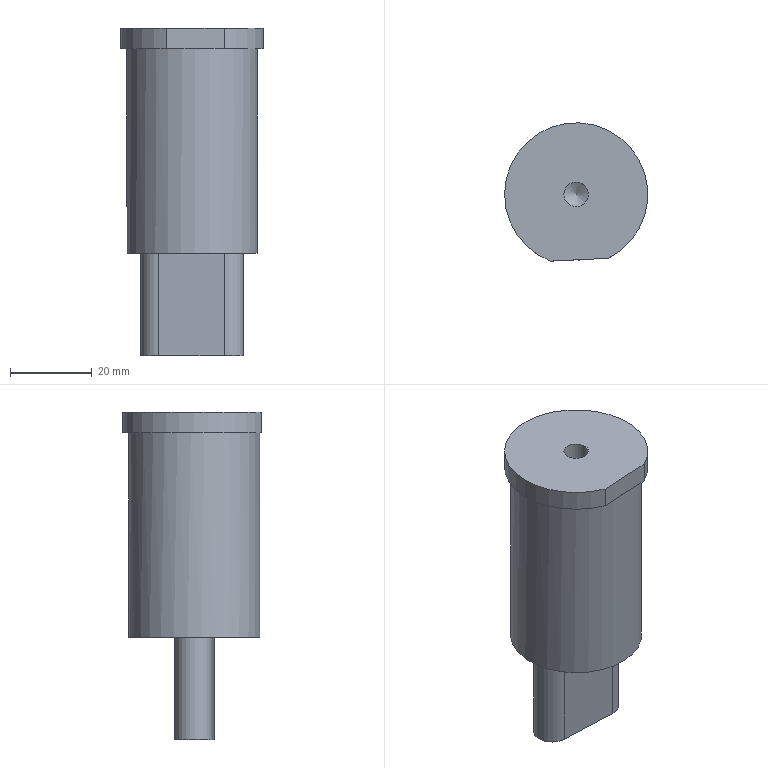Part | NX | features solid 2 | 1 solid | 13 faces | box 35 x 33.827 x 80 mm | volume 49834 mm3 | plane 7 | cylinder 5 | cone 1 | commonest cylinder face diameters 9.1 x2 6 x1 32 x1 35 x1
STEP:
#1=CARTESIAN_POINT('',(-48.126,272.664,48.));
#2=VERTEX_POINT('',#1);
#3=CARTESIAN_POINT('',(-48.741,256.676,48.));
#4=DIRECTION('',(0.,0.,1.));
#5=DIRECTION('',(0.03843,0.9993,0.));
#6=AXIS2_PLACEMENT_3D('',#3,#4,#5);
#7=CIRCLE('',#6,16.);
#8=EDGE_CURVE('',#2,#2,#7,.T.);
#9=ORIENTED_EDGE('',*,*,#8,.F.);
#10=EDGE_LOOP('',(#9));
#11=FACE_BOUND('',#10,.T.);
#12=CARTESIAN_POINT('',(-56.56,261.53,48.));
#13=VERTEX_POINT('',#12);
#14=CARTESIAN_POINT('',(-40.572,260.915,48.));
#15=VERTEX_POINT('',#14);
#16=CARTESIAN_POINT('',(-48.566,261.223,48.));
#17=DIRECTION('',(0.9993,-0.03843,0.));
#18=VECTOR('',#17,1000.);
#19=LINE('',#16,#18);
#20=EDGE_CURVE('',#13,#15,#19,.T.);
#21=ORIENTED_EDGE('',*,*,#20,.F.);
#22=CARTESIAN_POINT('',(-56.91,252.437,48.));
#23=VERTEX_POINT('',#22);
#24=CARTESIAN_POINT('',(-56.735,256.984,48.));
#25=DIRECTION('',(0.,0.,1.));
#26=DIRECTION('',(0.03843,0.9993,0.));
#27=AXIS2_PLACEMENT_3D('',#24,#25,#26);
#28=CIRCLE('',#27,4.55);
#29=EDGE_CURVE('',#13,#23,#28,.T.);
#30=ORIENTED_EDGE('',*,*,#29,.T.);
#31=CARTESIAN_POINT('',(-40.922,251.822,48.));
#32=VERTEX_POINT('',#31);
#33=CARTESIAN_POINT('',(-48.916,252.129,48.));
#34=DIRECTION('',(0.9993,-0.03843,0.));
#35=VECTOR('',#34,1000.);
#36=LINE('',#33,#35);
#37=EDGE_CURVE('',#23,#32,#36,.T.);
#38=ORIENTED_EDGE('',*,*,#37,.T.);
#39=CARTESIAN_POINT('',(-40.747,256.369,48.));
#40=DIRECTION('',(0.,0.,1.));
#41=DIRECTION('',(0.03843,0.9993,0.));
#42=AXIS2_PLACEMENT_3D('',#39,#40,#41);
#43=CIRCLE('',#42,4.55);
#44=EDGE_CURVE('',#32,#15,#43,.T.);
#45=ORIENTED_EDGE('',*,*,#44,.T.);
#46=EDGE_LOOP('',(#21,#30,#38,#45));
#47=FACE_BOUND('',#46,.T.);
#48=CARTESIAN_POINT('',(-48.741,256.676,48.));
#49=DIRECTION('',(0.,0.,1.));
#50=DIRECTION('',(0.03843,0.9993,0.));
#51=AXIS2_PLACEMENT_3D('',#48,#49,#50);
#52=PLANE('',#51);
#53=ADVANCED_FACE('',(#11,#47),#52,.F.);
#54=ORIENTED_EDGE('',*,*,#8,.T.);
#55=EDGE_LOOP('',(#54));
#56=FACE_BOUND('',#55,.T.);
#57=CARTESIAN_POINT('',(-47.96,240.695,98.));
#58=VERTEX_POINT('',#57);
#59=CARTESIAN_POINT('',(-48.741,256.676,98.));
#60=DIRECTION('',(0.,0.,1.));
#61=DIRECTION('',(-0.04881,0.9988,0.));
#62=AXIS2_PLACEMENT_3D('',#59,#60,#61);
#63=CIRCLE('',#62,16.);
#64=EDGE_CURVE('',#58,#58,#63,.T.);
#65=ORIENTED_EDGE('',*,*,#64,.F.);
#66=EDGE_LOOP('',(#65));
#67=FACE_BOUND('',#66,.T.);
#68=CARTESIAN_POINT('',(-48.741,256.676,103.));
#69=DIRECTION('',(0.,0.,-1.));
#70=DIRECTION('',(-0.03843,-0.9993,0.));
#71=AXIS2_PLACEMENT_3D('',#68,#69,#70);
#72=CYLINDRICAL_SURFACE('',#71,16.);
#73=ADVANCED_FACE('',(#56,#67),#72,.T.);
#74=CARTESIAN_POINT('',(-40.88,241.041,98.));
#75=VERTEX_POINT('',#74);
#76=CARTESIAN_POINT('',(-55.04,240.349,98.));
#77=VERTEX_POINT('',#76);
#78=CARTESIAN_POINT('',(-48.741,256.676,98.));
#79=DIRECTION('',(0.,0.,1.));
#80=DIRECTION('',(-0.04881,0.9988,0.));
#81=AXIS2_PLACEMENT_3D('',#78,#79,#80);
#82=CIRCLE('',#81,17.5);
#83=EDGE_CURVE('',#75,#77,#82,.T.);
#84=ORIENTED_EDGE('',*,*,#83,.F.);
#85=CARTESIAN_POINT('',(-47.96,240.695,98.));
#86=DIRECTION('',(-0.9988,-0.04881,0.));
#87=VECTOR('',#86,1000.);
#88=LINE('',#85,#87);
#89=EDGE_CURVE('',#75,#58,#88,.T.);
#90=ORIENTED_EDGE('',*,*,#89,.T.);
#91=ORIENTED_EDGE('',*,*,#64,.T.);
#92=CARTESIAN_POINT('',(-47.96,240.695,98.));
#93=DIRECTION('',(-0.9988,-0.04881,0.));
#94=VECTOR('',#93,1000.);
#95=LINE('',#92,#94);
#96=EDGE_CURVE('',#58,#77,#95,.T.);
#97=ORIENTED_EDGE('',*,*,#96,.T.);
#98=EDGE_LOOP('',(#84,#90,#91,#97));
#99=FACE_BOUND('',#98,.T.);
#100=CARTESIAN_POINT('',(-48.741,256.676,98.));
#101=DIRECTION('',(0.,0.,1.));
#102=DIRECTION('',(-0.04881,0.9988,0.));
#103=AXIS2_PLACEMENT_3D('',#100,#101,#102);
#104=PLANE('',#103);
#105=ADVANCED_FACE('',(#99),#104,.F.);
#106=CARTESIAN_POINT('',(-55.04,240.349,103.));
#107=VERTEX_POINT('',#106);
#108=CARTESIAN_POINT('',(-55.04,240.349,107.));
#109=DIRECTION('',(0.,0.,-1.));
#110=VECTOR('',#109,1000.);
#111=LINE('',#108,#110);
#112=EDGE_CURVE('',#107,#77,#111,.T.);
#113=ORIENTED_EDGE('',*,*,#112,.F.);
#114=CARTESIAN_POINT('',(-40.88,241.041,103.));
#115=VERTEX_POINT('',#114);
#116=CARTESIAN_POINT('',(-48.741,256.676,103.));
#117=DIRECTION('',(0.,0.,1.));
#118=DIRECTION('',(-0.04881,0.9988,0.));
#119=AXIS2_PLACEMENT_3D('',#116,#117,#118);
#120=CIRCLE('',#119,17.5);
#121=EDGE_CURVE('',#115,#107,#120,.T.);
#122=ORIENTED_EDGE('',*,*,#121,.F.);
#123=CARTESIAN_POINT('',(-40.88,241.041,107.));
#124=DIRECTION('',(0.,0.,-1.));
#125=VECTOR('',#124,1000.);
#126=LINE('',#123,#125);
#127=EDGE_CURVE('',#75,#115,#126,.F.);
#128=ORIENTED_EDGE('',*,*,#127,.F.);
#129=ORIENTED_EDGE('',*,*,#83,.T.);
#130=EDGE_LOOP('',(#113,#122,#128,#129));
#131=FACE_BOUND('',#130,.T.);
#132=CARTESIAN_POINT('',(-48.741,256.676,98.));
#133=DIRECTION('',(0.,0.,1.));
#134=DIRECTION('',(-0.04881,0.9988,0.));
#135=AXIS2_PLACEMENT_3D('',#132,#133,#134);
#136=CYLINDRICAL_SURFACE('',#135,17.5);
#137=ADVANCED_FACE('',(#131),#136,.T.);
#138=CARTESIAN_POINT('',(-48.594,253.68,103.));
#139=VERTEX_POINT('',#138);
#140=CARTESIAN_POINT('',(-48.741,256.676,103.));
#141=DIRECTION('',(0.,0.,-1.));
#142=DIRECTION('',(0.04881,-0.9988,0.));
#143=AXIS2_PLACEMENT_3D('',#140,#141,#142);
#144=CIRCLE('',#143,3.);
#145=EDGE_CURVE('',#139,#139,#144,.T.);
#146=ORIENTED_EDGE('',*,*,#145,.T.);
#147=EDGE_LOOP('',(#146));
#148=FACE_BOUND('',#147,.T.);
#149=CARTESIAN_POINT('',(-47.96,240.695,103.));
#150=DIRECTION('',(-0.9988,-0.04881,0.));
#151=VECTOR('',#150,1000.);
#152=LINE('',#149,#151);
#153=EDGE_CURVE('',#115,#107,#152,.T.);
#154=ORIENTED_EDGE('',*,*,#153,.F.);
#155=ORIENTED_EDGE('',*,*,#121,.T.);
#156=EDGE_LOOP('',(#154,#155));
#157=FACE_BOUND('',#156,.T.);
#158=CARTESIAN_POINT('',(-48.741,256.676,103.));
#159=DIRECTION('',(0.,0.,1.));
#160=DIRECTION('',(-0.04881,0.9988,0.));
#161=AXIS2_PLACEMENT_3D('',#158,#159,#160);
#162=PLANE('',#161);
#163=ADVANCED_FACE('',(#148,#157),#162,.T.);
#164=ORIENTED_EDGE('',*,*,#127,.T.);
#165=ORIENTED_EDGE('',*,*,#153,.T.);
#166=ORIENTED_EDGE('',*,*,#112,.T.);
#167=ORIENTED_EDGE('',*,*,#96,.F.);
#168=ORIENTED_EDGE('',*,*,#89,.F.);
#169=EDGE_LOOP('',(#164,#165,#166,#167,#168));
#170=FACE_BOUND('',#169,.T.);
#171=CARTESIAN_POINT('',(-55.04,240.349,107.));
#172=DIRECTION('',(-0.04881,0.9988,0.));
#173=DIRECTION('',(0.,0.,-1.));
#174=AXIS2_PLACEMENT_3D('',#171,#172,#173);
#175=PLANE('',#174);
#176=ADVANCED_FACE('',(#170),#175,.F.);
#177=CARTESIAN_POINT('',(-56.56,261.53,23.));
#178=VERTEX_POINT('',#177);
#179=CARTESIAN_POINT('',(-56.56,261.53,23.));
#180=DIRECTION('',(0.,0.,1.));
#181=VECTOR('',#180,1000.);
#182=LINE('',#179,#181);
#183=EDGE_CURVE('',#178,#13,#182,.T.);
#184=ORIENTED_EDGE('',*,*,#183,.T.);
#185=ORIENTED_EDGE('',*,*,#20,.T.);
#186=CARTESIAN_POINT('',(-40.572,260.915,23.));
#187=VERTEX_POINT('',#186);
#188=CARTESIAN_POINT('',(-40.572,260.915,23.));
#189=DIRECTION('',(0.,0.,1.));
#190=VECTOR('',#189,1000.);
#191=LINE('',#188,#190);
#192=EDGE_CURVE('',#187,#15,#191,.T.);
#193=ORIENTED_EDGE('',*,*,#192,.F.);
#194=CARTESIAN_POINT('',(-56.56,261.53,23.));
#195=DIRECTION('',(0.9993,-0.03843,0.));
#196=VECTOR('',#195,1000.);
#197=LINE('',#194,#196);
#198=EDGE_CURVE('',#178,#187,#197,.T.);
#199=ORIENTED_EDGE('',*,*,#198,.F.);
#200=EDGE_LOOP('',(#184,#185,#193,#199));
#201=FACE_BOUND('',#200,.T.);
#202=CARTESIAN_POINT('',(-56.56,261.53,23.));
#203=DIRECTION('',(-0.03843,-0.9993,0.));
#204=DIRECTION('',(0.,0.,1.));
#205=AXIS2_PLACEMENT_3D('',#202,#203,#204);
#206=PLANE('',#205);
#207=ADVANCED_FACE('',(#201),#206,.F.);
#208=ORIENTED_EDGE('',*,*,#44,.F.);
#209=CARTESIAN_POINT('',(-40.922,251.822,23.));
#210=VERTEX_POINT('',#209);
#211=CARTESIAN_POINT('',(-40.922,251.822,23.));
#212=DIRECTION('',(0.,0.,1.));
#213=VECTOR('',#212,1000.);
#214=LINE('',#211,#213);
#215=EDGE_CURVE('',#210,#32,#214,.T.);
#216=ORIENTED_EDGE('',*,*,#215,.F.);
#217=CARTESIAN_POINT('',(-40.747,256.369,23.));
#218=DIRECTION('',(0.,0.,1.));
#219=DIRECTION('',(0.03843,0.9993,0.));
#220=AXIS2_PLACEMENT_3D('',#217,#218,#219);
#221=CIRCLE('',#220,4.55);
#222=EDGE_CURVE('',#210,#187,#221,.T.);
#223=ORIENTED_EDGE('',*,*,#222,.T.);
#224=ORIENTED_EDGE('',*,*,#192,.T.);
#225=EDGE_LOOP('',(#208,#216,#223,#224));
#226=FACE_BOUND('',#225,.T.);
#227=CARTESIAN_POINT('',(-40.747,256.369,23.));
#228=DIRECTION('',(0.,0.,1.));
#229=DIRECTION('',(0.03843,0.9993,0.));
#230=AXIS2_PLACEMENT_3D('',#227,#228,#229);
#231=CYLINDRICAL_SURFACE('',#230,4.55);
#232=ADVANCED_FACE('',(#226),#231,.T.);
#233=ORIENTED_EDGE('',*,*,#37,.F.);
#234=CARTESIAN_POINT('',(-56.91,252.437,23.));
#235=VERTEX_POINT('',#234);
#236=CARTESIAN_POINT('',(-56.91,252.437,23.));
#237=DIRECTION('',(0.,0.,1.));
#238=VECTOR('',#237,1000.);
#239=LINE('',#236,#238);
#240=EDGE_CURVE('',#235,#23,#239,.T.);
#241=ORIENTED_EDGE('',*,*,#240,.F.);
#242=CARTESIAN_POINT('',(-56.91,252.437,23.));
#243=DIRECTION('',(0.9993,-0.03843,0.));
#244=VECTOR('',#243,1000.);
#245=LINE('',#242,#244);
#246=EDGE_CURVE('',#235,#210,#245,.T.);
#247=ORIENTED_EDGE('',*,*,#246,.T.);
#248=ORIENTED_EDGE('',*,*,#215,.T.);
#249=EDGE_LOOP('',(#233,#241,#247,#248));
#250=FACE_BOUND('',#249,.T.);
#251=CARTESIAN_POINT('',(-56.91,252.437,23.));
#252=DIRECTION('',(-0.03843,-0.9993,0.));
#253=DIRECTION('',(0.,0.,1.));
#254=AXIS2_PLACEMENT_3D('',#251,#252,#253);
#255=PLANE('',#254);
#256=ADVANCED_FACE('',(#250),#255,.T.);
#257=ORIENTED_EDGE('',*,*,#29,.F.);
#258=ORIENTED_EDGE('',*,*,#183,.F.);
#259=CARTESIAN_POINT('',(-56.735,256.984,23.));
#260=DIRECTION('',(0.,0.,1.));
#261=DIRECTION('',(0.03843,0.9993,0.));
#262=AXIS2_PLACEMENT_3D('',#259,#260,#261);
#263=CIRCLE('',#262,4.55);
#264=EDGE_CURVE('',#178,#235,#263,.T.);
#265=ORIENTED_EDGE('',*,*,#264,.T.);
#266=ORIENTED_EDGE('',*,*,#240,.T.);
#267=EDGE_LOOP('',(#257,#258,#265,#266));
#268=FACE_BOUND('',#267,.T.);
#269=CARTESIAN_POINT('',(-56.735,256.984,23.));
#270=DIRECTION('',(0.,0.,1.));
#271=DIRECTION('',(0.03843,0.9993,0.));
#272=AXIS2_PLACEMENT_3D('',#269,#270,#271);
#273=CYLINDRICAL_SURFACE('',#272,4.55);
#274=ADVANCED_FACE('',(#268),#273,.T.);
#275=ORIENTED_EDGE('',*,*,#198,.T.);
#276=ORIENTED_EDGE('',*,*,#222,.F.);
#277=ORIENTED_EDGE('',*,*,#246,.F.);
#278=ORIENTED_EDGE('',*,*,#264,.F.);
#279=EDGE_LOOP('',(#275,#276,#277,#278));
#280=FACE_BOUND('',#279,.T.);
#281=CARTESIAN_POINT('',(-40.747,256.369,23.));
#282=DIRECTION('',(0.,0.,1.));
#283=DIRECTION('',(0.03843,0.9993,0.));
#284=AXIS2_PLACEMENT_3D('',#281,#282,#283);
#285=PLANE('',#284);
#286=ADVANCED_FACE('',(#280),#285,.F.);
#287=CARTESIAN_POINT('',(-48.594,253.68,90.));
#288=VERTEX_POINT('',#287);
#289=CARTESIAN_POINT('',(-48.741,256.676,90.));
#290=DIRECTION('',(0.,0.,-1.));
#291=DIRECTION('',(0.04881,-0.9988,0.));
#292=AXIS2_PLACEMENT_3D('',#289,#290,#291);
#293=CIRCLE('',#292,3.);
#294=EDGE_CURVE('',#288,#288,#293,.T.);
#295=ORIENTED_EDGE('',*,*,#294,.F.);
#296=EDGE_LOOP('',(#295));
#297=FACE_BOUND('',#296,.T.);
#298=CARTESIAN_POINT('',(-48.741,256.676,88.268));
#299=VERTEX_POINT('',#298);
#300=VERTEX_LOOP('',#299);
#301=FACE_BOUND('',#300,.T.);
#302=CARTESIAN_POINT('',(-48.741,256.676,90.));
#303=DIRECTION('',(0.,0.,1.));
#304=DIRECTION('',(-0.04881,0.9988,0.));
#305=AXIS2_PLACEMENT_3D('',#302,#303,#304);
#306=CONICAL_SURFACE('',#305,3.,1.047);
#307=ADVANCED_FACE('',(#297,#301),#306,.F.);
#308=ORIENTED_EDGE('',*,*,#294,.T.);
#309=EDGE_LOOP('',(#308));
#310=FACE_BOUND('',#309,.T.);
#311=ORIENTED_EDGE('',*,*,#145,.F.);
#312=EDGE_LOOP('',(#311));
#313=FACE_BOUND('',#312,.T.);
#314=CARTESIAN_POINT('',(-48.741,256.676,103.));
#315=DIRECTION('',(0.,0.,-1.));
#316=DIRECTION('',(0.04881,-0.9988,0.));
#317=AXIS2_PLACEMENT_3D('',#314,#315,#316);
#318=CYLINDRICAL_SURFACE('',#317,3.);
#319=ADVANCED_FACE('',(#310,#313),#318,.F.);
#320=CLOSED_SHELL('',(#53,#73,#105,#137,#163,#176,#207,#232,#256,#274,#286,#307,#319));
#321=MANIFOLD_SOLID_BREP('',#320);
#322=(LENGTH_UNIT()NAMED_UNIT(*)SI_UNIT(.MILLI.,.METRE.));
#323=UNCERTAINTY_MEASURE_WITH_UNIT(LENGTH_MEASURE(0.00001),#322,'','');
#324=(NAMED_UNIT(*)PLANE_ANGLE_UNIT()SI_UNIT($,.RADIAN.));
#325=(NAMED_UNIT(*)SI_UNIT($,.STERADIAN.)SOLID_ANGLE_UNIT());
#326=(GEOMETRIC_REPRESENTATION_CONTEXT(3)GLOBAL_UNCERTAINTY_ASSIGNED_CONTEXT((#323))GLOBAL_UNIT_ASSIGNED_CONTEXT((#322,#324,#325))REPRESENTATION_CONTEXT('',''));
#327=ADVANCED_BREP_SHAPE_REPRESENTATION('',(#321),#326);